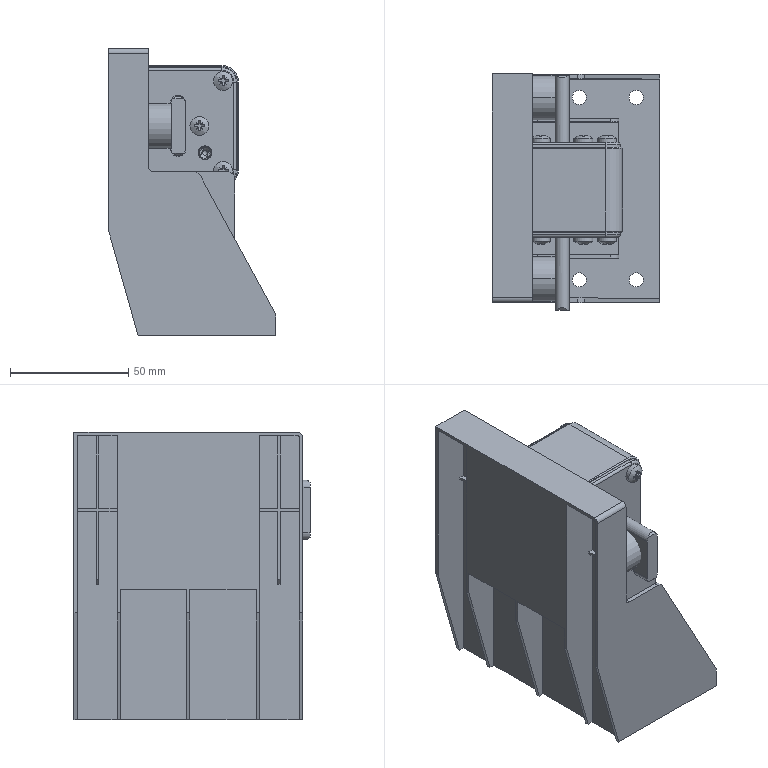Part | NX | features BREP 26 | 26 solids | 1170 faces | box 70.8 x 99.662 x 121.2 mm | volume 149161 mm3 | plane 696 | cylinder 385 | cone 57 | sphere 16 | torus 16 | commonest cylinder face diameters 4 x53 1.6 x48 5 x40 8 x32 6 x29 3.4 x24